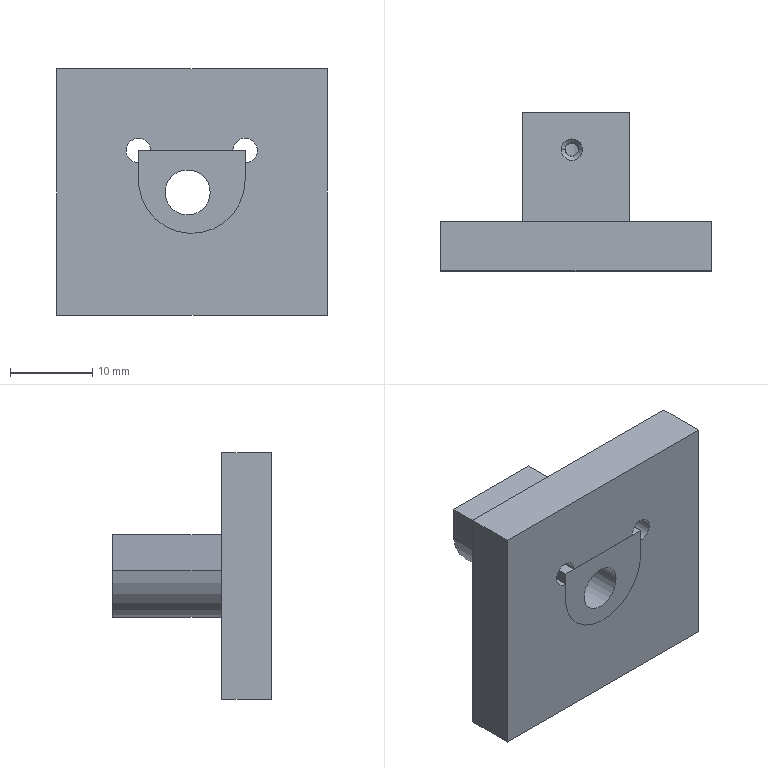Part | NX | 2 solids | 30 faces | box 32.951 x 19.3 x 30.1 mm | volume 6919 mm3 | plane 14 | cylinder 10 | cone 6 | commonest cylinder face diameters 1.6 x4 3 x2 5.5 x2 13 x2
STEP:
#1=CARTESIAN_POINT('',(-6.5,9.65,0.));
#2=VERTEX_POINT('',#1);
#3=CARTESIAN_POINT('',(-6.5,-9.65,0.));
#4=VERTEX_POINT('',#3);
#5=CARTESIAN_POINT('',(-6.5,9.65,0.));
#6=DIRECTION('',(0.,-1.,0.));
#7=VECTOR('',#6,1000.);
#8=LINE('',#5,#7);
#9=EDGE_CURVE('',#2,#4,#8,.T.);
#10=ORIENTED_EDGE('',*,*,#9,.F.);
#11=CARTESIAN_POINT('',(-6.451,9.65,-4.395));
#12=VERTEX_POINT('',#11);
#13=CARTESIAN_POINT('',(-2.87,9.65,-328.33));
#14=DIRECTION('',(0.01106,0.,-0.9999));
#15=VECTOR('',#14,1000.);
#16=LINE('',#13,#15);
#17=EDGE_CURVE('',#2,#12,#16,.T.);
#18=ORIENTED_EDGE('',*,*,#17,.T.);
#19=CARTESIAN_POINT('',(-6.451,-9.65,-4.395));
#20=VERTEX_POINT('',#19);
#21=CARTESIAN_POINT('',(-6.451,9.65,-4.395));
#22=CARTESIAN_POINT('',(-6.451,3.217,-4.395));
#23=CARTESIAN_POINT('',(-6.451,-3.217,-4.395));
#24=CARTESIAN_POINT('',(-6.451,-9.65,-4.395));
#25=B_SPLINE_CURVE_WITH_KNOTS('',3,(#21,#22,#23,#24),.UNSPECIFIED.,.F.,.F.,(4,4),(0.,1.),.UNSPECIFIED.);
#26=EDGE_CURVE('',#20,#12,#25,.F.);
#27=ORIENTED_EDGE('',*,*,#26,.F.);
#28=CARTESIAN_POINT('',(-6.462,-9.65,-3.4));
#29=DIRECTION('',(-0.01106,0.,0.9999));
#30=VECTOR('',#29,1000.);
#31=LINE('',#28,#30);
#32=EDGE_CURVE('',#20,#4,#31,.T.);
#33=ORIENTED_EDGE('',*,*,#32,.T.);
#34=EDGE_LOOP('',(#10,#18,#27,#33));
#35=FACE_BOUND('',#34,.T.);
#36=CARTESIAN_POINT('',(-6.5,-9.65,0.));
#37=DIRECTION('',(-0.9999,0.,-0.01106));
#38=DIRECTION('',(-0.01106,0.,0.9999));
#39=AXIS2_PLACEMENT_3D('',#36,#37,#38);
#40=PLANE('',#39);
#41=ADVANCED_FACE('',(#35),#40,.T.);
#42=ORIENTED_EDGE('',*,*,#32,.F.);
#43=CARTESIAN_POINT('',(6.5,-9.65,-3.6));
#44=VERTEX_POINT('',#43);
#45=CARTESIAN_POINT('',(0.,-9.65,-3.6));
#46=DIRECTION('',(0.,1.,0.));
#47=DIRECTION('',(1.,0.,-0.00002521));
#48=AXIS2_PLACEMENT_3D('',#45,#46,#47);
#49=CIRCLE('',#48,6.5);
#50=EDGE_CURVE('',#44,#20,#49,.T.);
#51=ORIENTED_EDGE('',*,*,#50,.F.);
#52=CARTESIAN_POINT('',(6.5,-9.65,0.));
#53=VERTEX_POINT('',#52);
#54=CARTESIAN_POINT('',(6.5,-9.65,0.));
#55=DIRECTION('',(0.,0.,-1.));
#56=VECTOR('',#55,1000.);
#57=LINE('',#54,#56);
#58=EDGE_CURVE('',#53,#44,#57,.T.);
#59=ORIENTED_EDGE('',*,*,#58,.F.);
#60=CARTESIAN_POINT('',(6.5,-9.65,0.));
#61=DIRECTION('',(-1.,0.,0.));
#62=VECTOR('',#61,1000.);
#63=LINE('',#60,#62);
#64=EDGE_CURVE('',#53,#4,#63,.T.);
#65=ORIENTED_EDGE('',*,*,#64,.T.);
#66=EDGE_LOOP('',(#42,#51,#59,#65));
#67=FACE_BOUND('',#66,.T.);
#68=CARTESIAN_POINT('',(2.25,-9.65,-5.1));
#69=VERTEX_POINT('',#68);
#70=CARTESIAN_POINT('',(-3.25,-9.65,-5.1));
#71=VERTEX_POINT('',#70);
#72=CARTESIAN_POINT('',(-0.5,-9.65,-5.1));
#73=DIRECTION('',(0.,-1.,0.));
#74=DIRECTION('',(1.,0.,0.));
#75=AXIS2_PLACEMENT_3D('',#72,#73,#74);
#76=CIRCLE('',#75,2.75);
#77=EDGE_CURVE('',#69,#71,#76,.T.);
#78=ORIENTED_EDGE('',*,*,#77,.F.);
#79=CARTESIAN_POINT('',(-0.5,-9.65,-5.1));
#80=DIRECTION('',(0.,-1.,0.));
#81=DIRECTION('',(-1.,0.,0.));
#82=AXIS2_PLACEMENT_3D('',#79,#80,#81);
#83=CIRCLE('',#82,2.75);
#84=EDGE_CURVE('',#71,#69,#83,.T.);
#85=ORIENTED_EDGE('',*,*,#84,.F.);
#86=EDGE_LOOP('',(#78,#85));
#87=FACE_BOUND('',#86,.T.);
#88=CARTESIAN_POINT('',(-6.5,-9.65,-3.4));
#89=DIRECTION('',(0.,1.,0.));
#90=DIRECTION('',(-1.,0.,0.));
#91=AXIS2_PLACEMENT_3D('',#88,#89,#90);
#92=PLANE('',#91);
#93=ADVANCED_FACE('',(#67,#87),#92,.F.);
#94=ORIENTED_EDGE('',*,*,#64,.F.);
#95=CARTESIAN_POINT('',(6.5,9.65,0.));
#96=VERTEX_POINT('',#95);
#97=CARTESIAN_POINT('',(6.5,-9.65,0.));
#98=DIRECTION('',(0.,1.,0.));
#99=VECTOR('',#98,1000.);
#100=LINE('',#97,#99);
#101=EDGE_CURVE('',#53,#96,#100,.T.);
#102=ORIENTED_EDGE('',*,*,#101,.T.);
#103=CARTESIAN_POINT('',(-6.5,9.65,0.));
#104=DIRECTION('',(1.,0.,0.));
#105=VECTOR('',#104,1000.);
#106=LINE('',#103,#105);
#107=EDGE_CURVE('',#2,#96,#106,.T.);
#108=ORIENTED_EDGE('',*,*,#107,.F.);
#109=ORIENTED_EDGE('',*,*,#9,.T.);
#110=EDGE_LOOP('',(#94,#102,#108,#109));
#111=FACE_BOUND('',#110,.T.);
#112=CARTESIAN_POINT('',(-0.5,-4.21,0.));
#113=VERTEX_POINT('',#112);
#114=CARTESIAN_POINT('',(-1.8,-5.51,0.));
#115=VERTEX_POINT('',#114);
#116=CARTESIAN_POINT('',(-0.5,-5.51,0.));
#117=DIRECTION('',(0.,0.,1.));
#118=DIRECTION('',(0.,1.,0.));
#119=AXIS2_PLACEMENT_3D('',#116,#117,#118);
#120=CIRCLE('',#119,1.3);
#121=EDGE_CURVE('',#113,#115,#120,.T.);
#122=ORIENTED_EDGE('',*,*,#121,.F.);
#123=CARTESIAN_POINT('',(0.8,-5.51,0.));
#124=VERTEX_POINT('',#123);
#125=CARTESIAN_POINT('',(-0.5,-5.51,0.));
#126=DIRECTION('',(0.,0.,1.));
#127=DIRECTION('',(1.,0.000000004,0.));
#128=AXIS2_PLACEMENT_3D('',#125,#126,#127);
#129=CIRCLE('',#128,1.3);
#130=EDGE_CURVE('',#124,#113,#129,.T.);
#131=ORIENTED_EDGE('',*,*,#130,.F.);
#132=CARTESIAN_POINT('',(-0.5,-6.81,0.));
#133=VERTEX_POINT('',#132);
#134=CARTESIAN_POINT('',(-0.5,-5.51,0.));
#135=DIRECTION('',(0.,0.,1.));
#136=DIRECTION('',(0.,-1.,0.));
#137=AXIS2_PLACEMENT_3D('',#134,#135,#136);
#138=CIRCLE('',#137,1.3);
#139=EDGE_CURVE('',#133,#124,#138,.T.);
#140=ORIENTED_EDGE('',*,*,#139,.F.);
#141=CARTESIAN_POINT('',(-0.5,-5.51,0.));
#142=DIRECTION('',(0.,0.,1.));
#143=DIRECTION('',(-1.,-0.000000004,0.));
#144=AXIS2_PLACEMENT_3D('',#141,#142,#143);
#145=CIRCLE('',#144,1.3);
#146=EDGE_CURVE('',#115,#133,#145,.T.);
#147=ORIENTED_EDGE('',*,*,#146,.F.);
#148=EDGE_LOOP('',(#122,#131,#140,#147));
#149=FACE_BOUND('',#148,.T.);
#150=CARTESIAN_POINT('',(-0.5,6.45,0.));
#151=VERTEX_POINT('',#150);
#152=CARTESIAN_POINT('',(-1.8,5.15,0.));
#153=VERTEX_POINT('',#152);
#154=CARTESIAN_POINT('',(-0.5,5.15,0.));
#155=DIRECTION('',(0.,0.,1.));
#156=DIRECTION('',(0.,1.,0.));
#157=AXIS2_PLACEMENT_3D('',#154,#155,#156);
#158=CIRCLE('',#157,1.3);
#159=EDGE_CURVE('',#151,#153,#158,.T.);
#160=ORIENTED_EDGE('',*,*,#159,.F.);
#161=CARTESIAN_POINT('',(0.8,5.15,0.));
#162=VERTEX_POINT('',#161);
#163=CARTESIAN_POINT('',(-0.5,5.15,0.));
#164=DIRECTION('',(0.,0.,1.));
#165=DIRECTION('',(1.,0.000000004,0.));
#166=AXIS2_PLACEMENT_3D('',#163,#164,#165);
#167=CIRCLE('',#166,1.3);
#168=EDGE_CURVE('',#162,#151,#167,.T.);
#169=ORIENTED_EDGE('',*,*,#168,.F.);
#170=CARTESIAN_POINT('',(-0.5,3.85,0.));
#171=VERTEX_POINT('',#170);
#172=CARTESIAN_POINT('',(-0.5,5.15,0.));
#173=DIRECTION('',(0.,0.,1.));
#174=DIRECTION('',(0.,-1.,0.));
#175=AXIS2_PLACEMENT_3D('',#172,#173,#174);
#176=CIRCLE('',#175,1.3);
#177=EDGE_CURVE('',#171,#162,#176,.T.);
#178=ORIENTED_EDGE('',*,*,#177,.F.);
#179=CARTESIAN_POINT('',(-0.5,5.15,0.));
#180=DIRECTION('',(0.,0.,1.));
#181=DIRECTION('',(-1.,-0.000000004,0.));
#182=AXIS2_PLACEMENT_3D('',#179,#180,#181);
#183=CIRCLE('',#182,1.3);
#184=EDGE_CURVE('',#153,#171,#183,.T.);
#185=ORIENTED_EDGE('',*,*,#184,.F.);
#186=EDGE_LOOP('',(#160,#169,#178,#185));
#187=FACE_BOUND('',#186,.T.);
#188=CARTESIAN_POINT('',(6.5,-9.65,0.));
#189=DIRECTION('',(0.,0.,1.));
#190=DIRECTION('',(1.,0.,0.));
#191=AXIS2_PLACEMENT_3D('',#188,#189,#190);
#192=PLANE('',#191);
#193=ADVANCED_FACE('',(#111,#149,#187),#192,.T.);
#194=CARTESIAN_POINT('',(6.5,9.65,-3.6));
#195=VERTEX_POINT('',#194);
#196=CARTESIAN_POINT('',(6.5,9.65,-3.6));
#197=DIRECTION('',(0.,0.000001693,1.));
#198=VECTOR('',#197,1000.);
#199=LINE('',#196,#198);
#200=EDGE_CURVE('',#195,#96,#199,.T.);
#201=ORIENTED_EDGE('',*,*,#200,.F.);
#202=CARTESIAN_POINT('',(0.,9.65,-3.6));
#203=DIRECTION('',(0.,-1.,0.));
#204=DIRECTION('',(-0.9925,0.,-0.1221));
#205=AXIS2_PLACEMENT_3D('',#202,#203,#204);
#206=CIRCLE('',#205,6.5);
#207=EDGE_CURVE('',#12,#195,#206,.T.);
#208=ORIENTED_EDGE('',*,*,#207,.F.);
#209=ORIENTED_EDGE('',*,*,#17,.F.);
#210=ORIENTED_EDGE('',*,*,#107,.T.);
#211=EDGE_LOOP('',(#201,#208,#209,#210));
#212=FACE_BOUND('',#211,.T.);
#213=CARTESIAN_POINT('',(2.75,9.65,-5.1));
#214=VERTEX_POINT('',#213);
#215=CARTESIAN_POINT('',(-3.75,9.65,-5.1));
#216=VERTEX_POINT('',#215);
#217=CARTESIAN_POINT('',(-0.5,9.65,-5.1));
#218=DIRECTION('',(0.,-1.,0.));
#219=DIRECTION('',(-1.,0.,0.));
#220=AXIS2_PLACEMENT_3D('',#217,#218,#219);
#221=CIRCLE('',#220,3.25);
#222=EDGE_CURVE('',#214,#216,#221,.F.);
#223=ORIENTED_EDGE('',*,*,#222,.F.);
#224=CARTESIAN_POINT('',(-0.5,9.65,-5.1));
#225=DIRECTION('',(0.,-1.,0.));
#226=DIRECTION('',(-1.,0.,0.));
#227=AXIS2_PLACEMENT_3D('',#224,#225,#226);
#228=CIRCLE('',#227,3.25);
#229=EDGE_CURVE('',#216,#214,#228,.F.);
#230=ORIENTED_EDGE('',*,*,#229,.F.);
#231=EDGE_LOOP('',(#223,#230));
#232=FACE_BOUND('',#231,.T.);
#233=CARTESIAN_POINT('',(126.5,9.65,-326.9));
#234=DIRECTION('',(0.,-1.,0.));
#235=DIRECTION('',(1.,0.,0.));
#236=AXIS2_PLACEMENT_3D('',#233,#234,#235);
#237=PLANE('',#236);
#238=ADVANCED_FACE('',(#212,#232),#237,.F.);
#239=ORIENTED_EDGE('',*,*,#207,.T.);
#240=CARTESIAN_POINT('',(6.5,-9.65,-3.6));
#241=DIRECTION('',(0.,1.,-0.000005657));
#242=VECTOR('',#241,1000.);
#243=LINE('',#240,#242);
#244=EDGE_CURVE('',#44,#195,#243,.T.);
#245=ORIENTED_EDGE('',*,*,#244,.F.);
#246=ORIENTED_EDGE('',*,*,#50,.T.);
#247=ORIENTED_EDGE('',*,*,#26,.T.);
#248=EDGE_LOOP('',(#239,#245,#246,#247));
#249=FACE_BOUND('',#248,.T.);
#250=CARTESIAN_POINT('',(0.,-730.231,-3.6));
#251=DIRECTION('',(0.,1.,0.));
#252=DIRECTION('',(-1.,0.,0.));
#253=AXIS2_PLACEMENT_3D('',#250,#251,#252);
#254=CYLINDRICAL_SURFACE('',#253,6.5);
#255=ADVANCED_FACE('',(#249),#254,.T.);
#256=ORIENTED_EDGE('',*,*,#58,.T.);
#257=ORIENTED_EDGE('',*,*,#244,.T.);
#258=ORIENTED_EDGE('',*,*,#200,.T.);
#259=ORIENTED_EDGE('',*,*,#101,.F.);
#260=EDGE_LOOP('',(#256,#257,#258,#259));
#261=FACE_BOUND('',#260,.T.);
#262=CARTESIAN_POINT('',(6.5,-166.75,-133.645));
#263=DIRECTION('',(-1.,0.,0.));
#264=DIRECTION('',(0.,-1.,0.));
#265=AXIS2_PLACEMENT_3D('',#262,#263,#264);
#266=PLANE('',#265);
#267=ADVANCED_FACE('',(#261),#266,.F.);
#268=CARTESIAN_POINT('',(-3.25,9.15,-5.1));
#269=VERTEX_POINT('',#268);
#270=CARTESIAN_POINT('',(-3.25,9.15,-5.1));
#271=CARTESIAN_POINT('',(-3.417,9.317,-5.1));
#272=CARTESIAN_POINT('',(-3.556,9.456,-5.1));
#273=CARTESIAN_POINT('',(-3.75,9.65,-5.1));
#274=B_SPLINE_CURVE_WITH_KNOTS('',3,(#270,#271,#272,#273),.UNSPECIFIED.,.F.,.F.,(4,4),(0.,0.9998),.UNSPECIFIED.);
#275=EDGE_CURVE('',#269,#216,#274,.T.);
#276=ORIENTED_EDGE('',*,*,#275,.T.);
#277=ORIENTED_EDGE('',*,*,#229,.T.);
#278=CARTESIAN_POINT('',(2.25,9.15,-5.1));
#279=VERTEX_POINT('',#278);
#280=CARTESIAN_POINT('',(2.75,9.65,-5.1));
#281=CARTESIAN_POINT('',(2.583,9.483,-5.1));
#282=CARTESIAN_POINT('',(2.416,9.317,-5.1));
#283=CARTESIAN_POINT('',(2.25,9.15,-5.1));
#284=B_SPLINE_CURVE_WITH_KNOTS('',3,(#280,#281,#282,#283),.UNSPECIFIED.,.F.,.F.,(4,4),(0.0001808,1.),.UNSPECIFIED.);
#285=EDGE_CURVE('',#214,#279,#284,.T.);
#286=ORIENTED_EDGE('',*,*,#285,.T.);
#287=CARTESIAN_POINT('',(-0.5,9.15,-5.1));
#288=DIRECTION('',(0.,1.,0.));
#289=DIRECTION('',(1.,0.,0.));
#290=AXIS2_PLACEMENT_3D('',#287,#288,#289);
#291=CIRCLE('',#290,2.75);
#292=EDGE_CURVE('',#269,#279,#291,.T.);
#293=ORIENTED_EDGE('',*,*,#292,.F.);
#294=EDGE_LOOP('',(#276,#277,#286,#293));
#295=FACE_BOUND('',#294,.T.);
#296=CARTESIAN_POINT('',(-0.5,9.4,-5.1));
#297=DIRECTION('',(0.,1.,0.));
#298=DIRECTION('',(-1.,0.,0.));
#299=AXIS2_PLACEMENT_3D('',#296,#297,#298);
#300=CONICAL_SURFACE('',#299,3.,0.7853);
#301=ADVANCED_FACE('',(#295),#300,.F.);
#302=CARTESIAN_POINT('',(2.25,-244.,-5.1));
#303=DIRECTION('',(0.,-1.,0.));
#304=VECTOR('',#303,1000.);
#305=LINE('',#302,#304);
#306=EDGE_CURVE('',#69,#279,#305,.F.);
#307=ORIENTED_EDGE('',*,*,#306,.F.);
#308=ORIENTED_EDGE('',*,*,#77,.T.);
#309=CARTESIAN_POINT('',(-3.25,-244.,-5.1));
#310=DIRECTION('',(0.,-1.,0.));
#311=VECTOR('',#310,1000.);
#312=LINE('',#309,#311);
#313=EDGE_CURVE('',#71,#269,#312,.F.);
#314=ORIENTED_EDGE('',*,*,#313,.T.);
#315=ORIENTED_EDGE('',*,*,#292,.T.);
#316=EDGE_LOOP('',(#307,#308,#314,#315));
#317=FACE_BOUND('',#316,.T.);
#318=CARTESIAN_POINT('',(-1.3,-5.51,-2.469));
#319=VERTEX_POINT('',#318);
#320=CARTESIAN_POINT('',(0.3,-5.51,-2.469));
#321=VERTEX_POINT('',#320);
#322=CARTESIAN_POINT('',(-1.3,-5.51,-2.469));
#323=CARTESIAN_POINT('',(-1.3,-5.085,-2.469));
#324=CARTESIAN_POINT('',(-0.5015,-4.336,-2.231));
#325=CARTESIAN_POINT('',(0.3,-5.085,-2.469));
#326=CARTESIAN_POINT('',(0.3,-5.51,-2.469));
#327=B_SPLINE_CURVE_WITH_KNOTS('',3,(#322,#323,#324,#325,#326),.UNSPECIFIED.,.F.,.F.,(4,1,4),(0.,0.001257,0.002514),.UNSPECIFIED.);
#328=EDGE_CURVE('',#319,#321,#327,.T.);
#329=ORIENTED_EDGE('',*,*,#328,.F.);
#330=CARTESIAN_POINT('',(0.3,-5.51,-2.469));
#331=CARTESIAN_POINT('',(0.3,-5.936,-2.469));
#332=CARTESIAN_POINT('',(-0.4985,-6.685,-2.231));
#333=CARTESIAN_POINT('',(-1.3,-5.936,-2.469));
#334=CARTESIAN_POINT('',(-1.3,-5.51,-2.469));
#335=B_SPLINE_CURVE_WITH_KNOTS('',3,(#330,#331,#332,#333,#334),.UNSPECIFIED.,.F.,.F.,(4,1,4),(0.,0.001257,0.002514),.UNSPECIFIED.);
#336=EDGE_CURVE('',#321,#319,#335,.T.);
#337=ORIENTED_EDGE('',*,*,#336,.F.);
#338=EDGE_LOOP('',(#329,#337));
#339=FACE_BOUND('',#338,.T.);
#340=CARTESIAN_POINT('',(-1.3,5.15,-2.469));
#341=VERTEX_POINT('',#340);
#342=CARTESIAN_POINT('',(0.3,5.15,-2.469));
#343=VERTEX_POINT('',#342);
#344=CARTESIAN_POINT('',(-1.3,5.15,-2.469));
#345=CARTESIAN_POINT('',(-1.3,5.575,-2.469));
#346=CARTESIAN_POINT('',(-0.5015,6.325,-2.231));
#347=CARTESIAN_POINT('',(0.3,5.575,-2.469));
#348=CARTESIAN_POINT('',(0.3,5.15,-2.469));
#349=B_SPLINE_CURVE_WITH_KNOTS('',3,(#344,#345,#346,#347,#348),.UNSPECIFIED.,.F.,.F.,(4,1,4),(0.,0.001257,0.002514),.UNSPECIFIED.);
#350=EDGE_CURVE('',#341,#343,#349,.T.);
#351=ORIENTED_EDGE('',*,*,#350,.F.);
#352=CARTESIAN_POINT('',(0.3,5.15,-2.469));
#353=CARTESIAN_POINT('',(0.3,4.725,-2.469));
#354=CARTESIAN_POINT('',(-0.4985,3.975,-2.231));
#355=CARTESIAN_POINT('',(-1.3,4.725,-2.469));
#356=CARTESIAN_POINT('',(-1.3,5.15,-2.469));
#357=B_SPLINE_CURVE_WITH_KNOTS('',3,(#352,#353,#354,#355,#356),.UNSPECIFIED.,.F.,.F.,(4,1,4),(0.,0.001257,0.002514),.UNSPECIFIED.);
#358=EDGE_CURVE('',#343,#341,#357,.T.);
#359=ORIENTED_EDGE('',*,*,#358,.F.);
#360=EDGE_LOOP('',(#351,#359));
#361=FACE_BOUND('',#360,.T.);
#362=CARTESIAN_POINT('',(-0.5,-244.,-5.1));
#363=DIRECTION('',(0.,-1.,0.));
#364=DIRECTION('',(1.,0.,0.));
#365=AXIS2_PLACEMENT_3D('',#362,#363,#364);
#366=CYLINDRICAL_SURFACE('',#365,2.75);
#367=ADVANCED_FACE('',(#317,#339,#361),#366,.F.);
#368=CARTESIAN_POINT('',(-0.5,9.15,-5.1));
#369=DIRECTION('',(0.,1.,0.));
#370=DIRECTION('',(1.,0.,0.));
#371=AXIS2_PLACEMENT_3D('',#368,#369,#370);
#372=CIRCLE('',#371,2.75);
#373=EDGE_CURVE('',#279,#269,#372,.T.);
#374=ORIENTED_EDGE('',*,*,#373,.T.);
#375=ORIENTED_EDGE('',*,*,#313,.F.);
#376=ORIENTED_EDGE('',*,*,#84,.T.);
#377=ORIENTED_EDGE('',*,*,#306,.T.);
#378=EDGE_LOOP('',(#374,#375,#376,#377));
#379=FACE_BOUND('',#378,.T.);
#380=CARTESIAN_POINT('',(-0.5,-244.,-5.1));
#381=DIRECTION('',(0.,-1.,0.));
#382=DIRECTION('',(1.,0.,0.));
#383=AXIS2_PLACEMENT_3D('',#380,#381,#382);
#384=CYLINDRICAL_SURFACE('',#383,2.75);
#385=ADVANCED_FACE('',(#379),#384,.F.);
#386=ORIENTED_EDGE('',*,*,#285,.F.);
#387=ORIENTED_EDGE('',*,*,#222,.T.);
#388=ORIENTED_EDGE('',*,*,#275,.F.);
#389=ORIENTED_EDGE('',*,*,#373,.F.);
#390=EDGE_LOOP('',(#386,#387,#388,#389));
#391=FACE_BOUND('',#390,.T.);
#392=CARTESIAN_POINT('',(-0.5,9.4,-5.1));
#393=DIRECTION('',(0.,1.,0.));
#394=DIRECTION('',(-1.,0.,0.));
#395=AXIS2_PLACEMENT_3D('',#392,#393,#394);
#396=CONICAL_SURFACE('',#395,3.,0.7853);
#397=ADVANCED_FACE('',(#391),#396,.F.);
#398=CARTESIAN_POINT('',(0.3,-5.51,-0.5));
#399=VERTEX_POINT('',#398);
#400=CARTESIAN_POINT('',(0.3,-5.51,-2.469));
#401=DIRECTION('',(0.000000004,0.000000196,1.));
#402=VECTOR('',#401,1000.);
#403=LINE('',#400,#402);
#404=EDGE_CURVE('',#399,#321,#403,.F.);
#405=ORIENTED_EDGE('',*,*,#404,.T.);
#406=ORIENTED_EDGE('',*,*,#336,.T.);
#407=CARTESIAN_POINT('',(-1.3,-5.51,-0.5));
#408=VERTEX_POINT('',#407);
#409=CARTESIAN_POINT('',(-1.3,-5.51,-2.469));
#410=DIRECTION('',(-0.000000004,-0.000000157,1.));
#411=VECTOR('',#410,1000.);
#412=LINE('',#409,#411);
#413=EDGE_CURVE('',#408,#319,#412,.F.);
#414=ORIENTED_EDGE('',*,*,#413,.F.);
#415=CARTESIAN_POINT('',(-0.5,-6.31,-0.5));
#416=VERTEX_POINT('',#415);
#417=CARTESIAN_POINT('',(-0.5,-5.51,-0.5));
#418=DIRECTION('',(0.,0.,1.));
#419=DIRECTION('',(-1.,0.,0.));
#420=AXIS2_PLACEMENT_3D('',#417,#418,#419);
#421=CIRCLE('',#420,0.8);
#422=EDGE_CURVE('',#408,#416,#421,.T.);
#423=ORIENTED_EDGE('',*,*,#422,.T.);
#424=CARTESIAN_POINT('',(-0.5,-5.51,-0.5));
#425=DIRECTION('',(0.,0.,1.));
#426=DIRECTION('',(0.,-1.,0.));
#427=AXIS2_PLACEMENT_3D('',#424,#425,#426);
#428=CIRCLE('',#427,0.8);
#429=EDGE_CURVE('',#416,#399,#428,.T.);
#430=ORIENTED_EDGE('',*,*,#429,.T.);
#431=EDGE_LOOP('',(#405,#406,#414,#423,#430));
#432=FACE_BOUND('',#431,.T.);
#433=CARTESIAN_POINT('',(-0.5,-5.51,1.1));
#434=DIRECTION('',(0.,0.,1.));
#435=DIRECTION('',(1.,0.,0.));
#436=AXIS2_PLACEMENT_3D('',#433,#434,#435);
#437=CYLINDRICAL_SURFACE('',#436,0.8);
#438=ADVANCED_FACE('',(#432),#437,.F.);
#439=CARTESIAN_POINT('',(0.8,-5.51,0.));
#440=DIRECTION('',(-0.7071,-0.000000331,-0.7071));
#441=VECTOR('',#440,1000.);
#442=LINE('',#439,#441);
#443=EDGE_CURVE('',#399,#124,#442,.F.);
#444=ORIENTED_EDGE('',*,*,#443,.F.);
#445=ORIENTED_EDGE('',*,*,#429,.F.);
#446=ORIENTED_EDGE('',*,*,#422,.F.);
#447=CARTESIAN_POINT('',(-1.8,-5.51,0.));
#448=DIRECTION('',(0.7071,0.000000005,-0.7071));
#449=VECTOR('',#448,1000.);
#450=LINE('',#447,#449);
#451=EDGE_CURVE('',#408,#115,#450,.F.);
#452=ORIENTED_EDGE('',*,*,#451,.T.);
#453=ORIENTED_EDGE('',*,*,#146,.T.);
#454=ORIENTED_EDGE('',*,*,#139,.T.);
#455=EDGE_LOOP('',(#444,#445,#446,#452,#453,#454));
#456=FACE_BOUND('',#455,.T.);
#457=CARTESIAN_POINT('',(-0.5,-5.51,-0.25));
#458=DIRECTION('',(0.,0.,1.));
#459=DIRECTION('',(0.,-1.,0.));
#460=AXIS2_PLACEMENT_3D('',#457,#458,#459);
#461=CONICAL_SURFACE('',#460,1.05,0.7854);
#462=ADVANCED_FACE('',(#456),#461,.F.);
#463=ORIENTED_EDGE('',*,*,#451,.F.);
#464=CARTESIAN_POINT('',(-0.5,-4.71,-0.5));
#465=VERTEX_POINT('',#464);
#466=CARTESIAN_POINT('',(-0.5,-5.51,-0.5));
#467=DIRECTION('',(0.,0.,1.));
#468=DIRECTION('',(0.,1.,0.));
#469=AXIS2_PLACEMENT_3D('',#466,#467,#468);
#470=CIRCLE('',#469,0.8);
#471=EDGE_CURVE('',#465,#408,#470,.T.);
#472=ORIENTED_EDGE('',*,*,#471,.F.);
#473=CARTESIAN_POINT('',(-0.5,-5.51,-0.5));
#474=DIRECTION('',(0.,0.,1.));
#475=DIRECTION('',(1.,-0.000000577,0.));
#476=AXIS2_PLACEMENT_3D('',#473,#474,#475);
#477=CIRCLE('',#476,0.8);
#478=EDGE_CURVE('',#399,#465,#477,.T.);
#479=ORIENTED_EDGE('',*,*,#478,.F.);
#480=ORIENTED_EDGE('',*,*,#443,.T.);
#481=ORIENTED_EDGE('',*,*,#130,.T.);
#482=ORIENTED_EDGE('',*,*,#121,.T.);
#483=EDGE_LOOP('',(#463,#472,#479,#480,#481,#482));
#484=FACE_BOUND('',#483,.T.);
#485=CARTESIAN_POINT('',(-0.5,-5.51,-0.25));
#486=DIRECTION('',(0.,0.,1.));
#487=DIRECTION('',(0.,-1.,0.));
#488=AXIS2_PLACEMENT_3D('',#485,#486,#487);
#489=CONICAL_SURFACE('',#488,1.05,0.7854);
#490=ADVANCED_FACE('',(#484),#489,.F.);
#491=ORIENTED_EDGE('',*,*,#413,.T.);
#492=ORIENTED_EDGE('',*,*,#328,.T.);
#493=ORIENTED_EDGE('',*,*,#404,.F.);
#494=ORIENTED_EDGE('',*,*,#478,.T.);
#495=ORIENTED_EDGE('',*,*,#471,.T.);
#496=EDGE_LOOP('',(#491,#492,#493,#494,#495));
#497=FACE_BOUND('',#496,.T.);
#498=CARTESIAN_POINT('',(-0.5,-5.51,1.1));
#499=DIRECTION('',(0.,0.,1.));
#500=DIRECTION('',(1.,0.,0.));
#501=AXIS2_PLACEMENT_3D('',#498,#499,#500);
#502=CYLINDRICAL_SURFACE('',#501,0.8);
#503=ADVANCED_FACE('',(#497),#502,.F.);
#504=CARTESIAN_POINT('',(0.3,5.15,-0.5));
#505=VERTEX_POINT('',#504);
#506=CARTESIAN_POINT('',(0.3,5.15,-2.469));
#507=DIRECTION('',(0.000000004,0.000000196,1.));
#508=VECTOR('',#507,1000.);
#509=LINE('',#506,#508);
#510=EDGE_CURVE('',#505,#343,#509,.F.);
#511=ORIENTED_EDGE('',*,*,#510,.T.);
#512=ORIENTED_EDGE('',*,*,#358,.T.);
#513=CARTESIAN_POINT('',(-1.3,5.15,-0.5));
#514=VERTEX_POINT('',#513);
#515=CARTESIAN_POINT('',(-1.3,5.15,-2.469));
#516=DIRECTION('',(-0.000000004,-0.000000157,1.));
#517=VECTOR('',#516,1000.);
#518=LINE('',#515,#517);
#519=EDGE_CURVE('',#514,#341,#518,.F.);
#520=ORIENTED_EDGE('',*,*,#519,.F.);
#521=CARTESIAN_POINT('',(-0.5,4.35,-0.5));
#522=VERTEX_POINT('',#521);
#523=CARTESIAN_POINT('',(-0.5,5.15,-0.5));
#524=DIRECTION('',(0.,0.,1.));
#525=DIRECTION('',(-1.,0.,0.));
#526=AXIS2_PLACEMENT_3D('',#523,#524,#525);
#527=CIRCLE('',#526,0.8);
#528=EDGE_CURVE('',#514,#522,#527,.T.);
#529=ORIENTED_EDGE('',*,*,#528,.T.);
#530=CARTESIAN_POINT('',(-0.5,5.15,-0.5));
#531=DIRECTION('',(0.,0.,1.));
#532=DIRECTION('',(0.,-1.,0.));
#533=AXIS2_PLACEMENT_3D('',#530,#531,#532);
#534=CIRCLE('',#533,0.8);
#535=EDGE_CURVE('',#522,#505,#534,.T.);
#536=ORIENTED_EDGE('',*,*,#535,.T.);
#537=EDGE_LOOP('',(#511,#512,#520,#529,#536));
#538=FACE_BOUND('',#537,.T.);
#539=CARTESIAN_POINT('',(-0.5,5.15,1.1));
#540=DIRECTION('',(0.,0.,1.));
#541=DIRECTION('',(1.,0.,0.));
#542=AXIS2_PLACEMENT_3D('',#539,#540,#541);
#543=CYLINDRICAL_SURFACE('',#542,0.8);
#544=ADVANCED_FACE('',(#538),#543,.F.);
#545=CARTESIAN_POINT('',(0.8,5.15,0.));
#546=DIRECTION('',(-0.7071,-0.000000331,-0.7071));
#547=VECTOR('',#546,1000.);
#548=LINE('',#545,#547);
#549=EDGE_CURVE('',#505,#162,#548,.F.);
#550=ORIENTED_EDGE('',*,*,#549,.F.);
#551=ORIENTED_EDGE('',*,*,#535,.F.);
#552=ORIENTED_EDGE('',*,*,#528,.F.);
#553=CARTESIAN_POINT('',(-1.8,5.15,0.));
#554=DIRECTION('',(0.7071,0.000000005,-0.7071));
#555=VECTOR('',#554,1000.);
#556=LINE('',#553,#555);
#557=EDGE_CURVE('',#514,#153,#556,.F.);
#558=ORIENTED_EDGE('',*,*,#557,.T.);
#559=ORIENTED_EDGE('',*,*,#184,.T.);
#560=ORIENTED_EDGE('',*,*,#177,.T.);
#561=EDGE_LOOP('',(#550,#551,#552,#558,#559,#560));
#562=FACE_BOUND('',#561,.T.);
#563=CARTESIAN_POINT('',(-0.5,5.15,-0.25));
#564=DIRECTION('',(0.,0.,1.));
#565=DIRECTION('',(0.,-1.,0.));
#566=AXIS2_PLACEMENT_3D('',#563,#564,#565);
#567=CONICAL_SURFACE('',#566,1.05,0.7854);
#568=ADVANCED_FACE('',(#562),#567,.F.);
#569=ORIENTED_EDGE('',*,*,#557,.F.);
#570=CARTESIAN_POINT('',(-0.5,5.95,-0.5));
#571=VERTEX_POINT('',#570);
#572=CARTESIAN_POINT('',(-0.5,5.15,-0.5));
#573=DIRECTION('',(0.,0.,1.));
#574=DIRECTION('',(0.,1.,0.));
#575=AXIS2_PLACEMENT_3D('',#572,#573,#574);
#576=CIRCLE('',#575,0.8);
#577=EDGE_CURVE('',#571,#514,#576,.T.);
#578=ORIENTED_EDGE('',*,*,#577,.F.);
#579=CARTESIAN_POINT('',(-0.5,5.15,-0.5));
#580=DIRECTION('',(0.,0.,1.));
#581=DIRECTION('',(1.,-0.000000577,0.));
#582=AXIS2_PLACEMENT_3D('',#579,#580,#581);
#583=CIRCLE('',#582,0.8);
#584=EDGE_CURVE('',#505,#571,#583,.T.);
#585=ORIENTED_EDGE('',*,*,#584,.F.);
#586=ORIENTED_EDGE('',*,*,#549,.T.);
#587=ORIENTED_EDGE('',*,*,#168,.T.);
#588=ORIENTED_EDGE('',*,*,#159,.T.);
#589=EDGE_LOOP('',(#569,#578,#585,#586,#587,#588));
#590=FACE_BOUND('',#589,.T.);
#591=CARTESIAN_POINT('',(-0.5,5.15,-0.25));
#592=DIRECTION('',(0.,0.,1.));
#593=DIRECTION('',(0.,-1.,0.));
#594=AXIS2_PLACEMENT_3D('',#591,#592,#593);
#595=CONICAL_SURFACE('',#594,1.05,0.7854);
#596=ADVANCED_FACE('',(#590),#595,.F.);
#597=ORIENTED_EDGE('',*,*,#519,.T.);
#598=ORIENTED_EDGE('',*,*,#350,.T.);
#599=ORIENTED_EDGE('',*,*,#510,.F.);
#600=ORIENTED_EDGE('',*,*,#584,.T.);
#601=ORIENTED_EDGE('',*,*,#577,.T.);
#602=EDGE_LOOP('',(#597,#598,#599,#600,#601));
#603=FACE_BOUND('',#602,.T.);
#604=CARTESIAN_POINT('',(-0.5,5.15,1.1));
#605=DIRECTION('',(0.,0.,1.));
#606=DIRECTION('',(1.,0.,0.));
#607=AXIS2_PLACEMENT_3D('',#604,#605,#606);
#608=CYLINDRICAL_SURFACE('',#607,0.8);
#609=ADVANCED_FACE('',(#603),#608,.F.);
#610=CLOSED_SHELL('',(#41,#93,#193,#238,#255,#267,#301,#367,#385,#397,#438,#462,#490,#503,#544,#568,#596,#609));
#611=MANIFOLD_SOLID_BREP('',#610);
#612=CARTESIAN_POINT('',(-6.451,-9.65,-4.395));
#613=VERTEX_POINT('',#612);
#614=CARTESIAN_POINT('',(6.5,-9.65,-3.6));
#615=VERTEX_POINT('',#614);
#616=CARTESIAN_POINT('',(0.,-9.65,-3.6));
#617=DIRECTION('',(0.,-1.,0.));
#618=DIRECTION('',(1.,0.,-0.00002521));
#619=AXIS2_PLACEMENT_3D('',#616,#617,#618);
#620=CIRCLE('',#619,6.5);
#621=EDGE_CURVE('',#613,#615,#620,.T.);
#622=ORIENTED_EDGE('',*,*,#621,.T.);
#623=CARTESIAN_POINT('',(6.5,-3.65,-3.6));
#624=VERTEX_POINT('',#623);
#625=CARTESIAN_POINT('',(6.5,-3.65,-3.6));
#626=DIRECTION('',(0.,-1.,0.));
#627=VECTOR('',#626,1000.);
#628=LINE('',#625,#627);
#629=EDGE_CURVE('',#624,#615,#628,.T.);
#630=ORIENTED_EDGE('',*,*,#629,.F.);
#631=CARTESIAN_POINT('',(-6.451,-3.65,-4.395));
#632=VERTEX_POINT('',#631);
#633=CARTESIAN_POINT('',(0.,-3.65,-3.6));
#634=DIRECTION('',(0.,-1.,0.));
#635=DIRECTION('',(1.,0.,-0.00002521));
#636=AXIS2_PLACEMENT_3D('',#633,#634,#635);
#637=CIRCLE('',#636,6.5);
#638=EDGE_CURVE('',#632,#624,#637,.T.);
#639=ORIENTED_EDGE('',*,*,#638,.F.);
#640=CARTESIAN_POINT('',(-6.451,-9.65,-4.395));
#641=CARTESIAN_POINT('',(-6.451,-7.65,-4.395));
#642=CARTESIAN_POINT('',(-6.451,-5.65,-4.395));
#643=CARTESIAN_POINT('',(-6.451,-3.65,-4.395));
#644=B_SPLINE_CURVE_WITH_KNOTS('',3,(#640,#641,#642,#643),.UNSPECIFIED.,.F.,.F.,(4,4),(0.,1.),.UNSPECIFIED.);
#645=EDGE_CURVE('',#632,#613,#644,.F.);
#646=ORIENTED_EDGE('',*,*,#645,.T.);
#647=EDGE_LOOP('',(#622,#630,#639,#646));
#648=FACE_BOUND('',#647,.T.);
#649=CARTESIAN_POINT('',(0.,-3.65,-3.6));
#650=DIRECTION('',(0.,-1.,0.));
#651=DIRECTION('',(0.,0.,-1.));
#652=AXIS2_PLACEMENT_3D('',#649,#650,#651);
#653=CYLINDRICAL_SURFACE('',#652,6.5);
#654=ADVANCED_FACE('',(#648),#653,.F.);
#655=CARTESIAN_POINT('',(6.5,-9.65,-1.5));
#656=VERTEX_POINT('',#655);
#657=CARTESIAN_POINT('',(6.5,-9.65,-3.6));
#658=DIRECTION('',(0.,0.,1.));
#659=VECTOR('',#658,1000.);
#660=LINE('',#657,#659);
#661=EDGE_CURVE('',#615,#656,#660,.T.);
#662=ORIENTED_EDGE('',*,*,#661,.T.);
#663=CARTESIAN_POINT('',(6.5,-3.65,-1.5));
#664=VERTEX_POINT('',#663);
#665=CARTESIAN_POINT('',(6.5,-3.65,-1.5));
#666=DIRECTION('',(0.,-1.,0.));
#667=VECTOR('',#666,1000.);
#668=LINE('',#665,#667);
#669=EDGE_CURVE('',#664,#656,#668,.T.);
#670=ORIENTED_EDGE('',*,*,#669,.F.);
#671=CARTESIAN_POINT('',(6.5,-3.65,-3.6));
#672=DIRECTION('',(0.,0.,1.));
#673=VECTOR('',#672,1000.);
#674=LINE('',#671,#673);
#675=EDGE_CURVE('',#624,#664,#674,.T.);
#676=ORIENTED_EDGE('',*,*,#675,.F.);
#677=ORIENTED_EDGE('',*,*,#629,.T.);
#678=EDGE_LOOP('',(#662,#670,#676,#677));
#679=FACE_BOUND('',#678,.T.);
#680=CARTESIAN_POINT('',(6.5,-3.65,-3.6));
#681=DIRECTION('',(1.,0.,0.));
#682=DIRECTION('',(0.,0.,-1.));
#683=AXIS2_PLACEMENT_3D('',#680,#681,#682);
#684=PLANE('',#683);
#685=ADVANCED_FACE('',(#679),#684,.F.);
#686=CARTESIAN_POINT('',(5.,-9.65,0.));
#687=VERTEX_POINT('',#686);
#688=CARTESIAN_POINT('',(6.5,-9.65,0.));
#689=DIRECTION('',(0.,-1.,0.));
#690=DIRECTION('',(0.,0.,-1.));
#691=AXIS2_PLACEMENT_3D('',#688,#689,#690);
#692=CIRCLE('',#691,1.5);
#693=EDGE_CURVE('',#656,#687,#692,.T.);
#694=ORIENTED_EDGE('',*,*,#693,.T.);
#695=CARTESIAN_POINT('',(5.,-3.65,0.));
#696=VERTEX_POINT('',#695);
#697=CARTESIAN_POINT('',(5.,-3.65,0.));
#698=DIRECTION('',(0.,-1.,0.));
#699=VECTOR('',#698,1000.);
#700=LINE('',#697,#699);
#701=EDGE_CURVE('',#696,#687,#700,.T.);
#702=ORIENTED_EDGE('',*,*,#701,.F.);
#703=CARTESIAN_POINT('',(6.5,-3.65,0.));
#704=DIRECTION('',(0.,-1.,0.));
#705=DIRECTION('',(0.,0.,-1.));
#706=AXIS2_PLACEMENT_3D('',#703,#704,#705);
#707=CIRCLE('',#706,1.5);
#708=EDGE_CURVE('',#664,#696,#707,.T.);
#709=ORIENTED_EDGE('',*,*,#708,.F.);
#710=ORIENTED_EDGE('',*,*,#669,.T.);
#711=EDGE_LOOP('',(#694,#702,#709,#710));
#712=FACE_BOUND('',#711,.T.);
#713=CARTESIAN_POINT('',(6.5,-3.65,0.));
#714=DIRECTION('',(0.,-1.,0.));
#715=DIRECTION('',(0.,0.,-1.));
#716=AXIS2_PLACEMENT_3D('',#713,#714,#715);
#717=CYLINDRICAL_SURFACE('',#716,1.5);
#718=ADVANCED_FACE('',(#712),#717,.F.);
#719=CARTESIAN_POINT('',(-5.,-9.65,0.));
#720=VERTEX_POINT('',#719);
#721=CARTESIAN_POINT('',(5.,-9.65,0.));
#722=DIRECTION('',(-1.,0.,0.));
#723=VECTOR('',#722,1000.);
#724=LINE('',#721,#723);
#725=EDGE_CURVE('',#687,#720,#724,.T.);
#726=ORIENTED_EDGE('',*,*,#725,.T.);
#727=CARTESIAN_POINT('',(-5.,-3.65,0.));
#728=VERTEX_POINT('',#727);
#729=CARTESIAN_POINT('',(-5.,-3.65,0.));
#730=DIRECTION('',(0.,-1.,0.));
#731=VECTOR('',#730,1000.);
#732=LINE('',#729,#731);
#733=EDGE_CURVE('',#728,#720,#732,.T.);
#734=ORIENTED_EDGE('',*,*,#733,.F.);
#735=CARTESIAN_POINT('',(5.,-3.65,0.));
#736=DIRECTION('',(-1.,0.,0.));
#737=VECTOR('',#736,1000.);
#738=LINE('',#735,#737);
#739=EDGE_CURVE('',#696,#728,#738,.T.);
#740=ORIENTED_EDGE('',*,*,#739,.F.);
#741=ORIENTED_EDGE('',*,*,#701,.T.);
#742=EDGE_LOOP('',(#726,#734,#740,#741));
#743=FACE_BOUND('',#742,.T.);
#744=CARTESIAN_POINT('',(5.,-3.65,0.));
#745=DIRECTION('',(0.,0.,1.));
#746=DIRECTION('',(1.,0.,0.));
#747=AXIS2_PLACEMENT_3D('',#744,#745,#746);
#748=PLANE('',#747);
#749=ADVANCED_FACE('',(#743),#748,.F.);
#750=CARTESIAN_POINT('',(-6.483,-9.65,-1.5));
#751=VERTEX_POINT('',#750);
#752=CARTESIAN_POINT('',(-6.5,-9.65,0.));
#753=DIRECTION('',(0.,-1.,0.));
#754=DIRECTION('',(0.,0.,-1.));
#755=AXIS2_PLACEMENT_3D('',#752,#753,#754);
#756=CIRCLE('',#755,1.5);
#757=EDGE_CURVE('',#720,#751,#756,.T.);
#758=ORIENTED_EDGE('',*,*,#757,.T.);
#759=CARTESIAN_POINT('',(-6.483,-3.65,-1.5));
#760=VERTEX_POINT('',#759);
#761=CARTESIAN_POINT('',(-6.483,-3.65,-1.5));
#762=DIRECTION('',(0.,-1.,0.));
#763=VECTOR('',#762,1000.);
#764=LINE('',#761,#763);
#765=EDGE_CURVE('',#760,#751,#764,.T.);
#766=ORIENTED_EDGE('',*,*,#765,.F.);
#767=CARTESIAN_POINT('',(-6.5,-3.65,0.));
#768=DIRECTION('',(0.,-1.,0.));
#769=DIRECTION('',(0.,0.,-1.));
#770=AXIS2_PLACEMENT_3D('',#767,#768,#769);
#771=CIRCLE('',#770,1.5);
#772=EDGE_CURVE('',#728,#760,#771,.T.);
#773=ORIENTED_EDGE('',*,*,#772,.F.);
#774=ORIENTED_EDGE('',*,*,#733,.T.);
#775=EDGE_LOOP('',(#758,#766,#773,#774));
#776=FACE_BOUND('',#775,.T.);
#777=CARTESIAN_POINT('',(-6.5,-3.65,0.));
#778=DIRECTION('',(0.,-1.,0.));
#779=DIRECTION('',(0.,0.,-1.));
#780=AXIS2_PLACEMENT_3D('',#777,#778,#779);
#781=CYLINDRICAL_SURFACE('',#780,1.5);
#782=ADVANCED_FACE('',(#776),#781,.F.);
#783=CARTESIAN_POINT('',(-16.451,-9.65,10.));
#784=VERTEX_POINT('',#783);
#785=CARTESIAN_POINT('',(16.5,-9.65,10.));
#786=VERTEX_POINT('',#785);
#787=CARTESIAN_POINT('',(-16.451,-9.65,10.));
#788=DIRECTION('',(1.,0.,0.));
#789=VECTOR('',#788,1000.);
#790=LINE('',#787,#789);
#791=EDGE_CURVE('',#784,#786,#790,.T.);
#792=ORIENTED_EDGE('',*,*,#791,.T.);
#793=CARTESIAN_POINT('',(16.5,-3.65,10.));
#794=VERTEX_POINT('',#793);
#795=CARTESIAN_POINT('',(16.5,-3.65,10.));
#796=DIRECTION('',(0.,-1.,0.));
#797=VECTOR('',#796,1000.);
#798=LINE('',#795,#797);
#799=EDGE_CURVE('',#794,#786,#798,.T.);
#800=ORIENTED_EDGE('',*,*,#799,.F.);
#801=CARTESIAN_POINT('',(-16.451,-3.65,10.));
#802=VERTEX_POINT('',#801);
#803=CARTESIAN_POINT('',(-16.451,-3.65,10.));
#804=DIRECTION('',(1.,0.,0.));
#805=VECTOR('',#804,1000.);
#806=LINE('',#803,#805);
#807=EDGE_CURVE('',#802,#794,#806,.T.);
#808=ORIENTED_EDGE('',*,*,#807,.F.);
#809=CARTESIAN_POINT('',(-16.451,-3.65,10.));
#810=DIRECTION('',(0.,-1.,0.));
#811=VECTOR('',#810,1000.);
#812=LINE('',#809,#811);
#813=EDGE_CURVE('',#802,#784,#812,.T.);
#814=ORIENTED_EDGE('',*,*,#813,.T.);
#815=EDGE_LOOP('',(#792,#800,#808,#814));
#816=FACE_BOUND('',#815,.T.);
#817=CARTESIAN_POINT('',(-16.451,-3.65,10.));
#818=DIRECTION('',(0.,0.,-1.));
#819=DIRECTION('',(-1.,0.,0.));
#820=AXIS2_PLACEMENT_3D('',#817,#818,#819);
#821=PLANE('',#820);
#822=ADVANCED_FACE('',(#816),#821,.F.);
#823=CARTESIAN_POINT('',(16.5,-9.65,-20.1));
#824=VERTEX_POINT('',#823);
#825=CARTESIAN_POINT('',(16.5,-9.65,10.));
#826=DIRECTION('',(0.,0.,-1.));
#827=VECTOR('',#826,1000.);
#828=LINE('',#825,#827);
#829=EDGE_CURVE('',#786,#824,#828,.T.);
#830=ORIENTED_EDGE('',*,*,#829,.T.);
#831=CARTESIAN_POINT('',(16.5,-3.65,-20.1));
#832=VERTEX_POINT('',#831);
#833=CARTESIAN_POINT('',(16.5,-3.65,-20.1));
#834=DIRECTION('',(0.,-1.,0.));
#835=VECTOR('',#834,1000.);
#836=LINE('',#833,#835);
#837=EDGE_CURVE('',#832,#824,#836,.T.);
#838=ORIENTED_EDGE('',*,*,#837,.F.);
#839=CARTESIAN_POINT('',(16.5,-3.65,10.));
#840=DIRECTION('',(0.,0.,-1.));
#841=VECTOR('',#840,1000.);
#842=LINE('',#839,#841);
#843=EDGE_CURVE('',#794,#832,#842,.T.);
#844=ORIENTED_EDGE('',*,*,#843,.F.);
#845=ORIENTED_EDGE('',*,*,#799,.T.);
#846=EDGE_LOOP('',(#830,#838,#844,#845));
#847=FACE_BOUND('',#846,.T.);
#848=CARTESIAN_POINT('',(16.5,-3.65,10.));
#849=DIRECTION('',(-1.,0.,0.));
#850=DIRECTION('',(0.,0.,1.));
#851=AXIS2_PLACEMENT_3D('',#848,#849,#850);
#852=PLANE('',#851);
#853=ADVANCED_FACE('',(#847),#852,.F.);
#854=CARTESIAN_POINT('',(-16.451,-9.65,-20.1));
#855=VERTEX_POINT('',#854);
#856=CARTESIAN_POINT('',(16.5,-9.65,-20.1));
#857=DIRECTION('',(-1.,0.,0.));
#858=VECTOR('',#857,1000.);
#859=LINE('',#856,#858);
#860=EDGE_CURVE('',#824,#855,#859,.T.);
#861=ORIENTED_EDGE('',*,*,#860,.T.);
#862=CARTESIAN_POINT('',(-16.451,-3.65,-20.1));
#863=VERTEX_POINT('',#862);
#864=CARTESIAN_POINT('',(-16.451,-3.65,-20.1));
#865=DIRECTION('',(0.,-1.,0.));
#866=VECTOR('',#865,1000.);
#867=LINE('',#864,#866);
#868=EDGE_CURVE('',#863,#855,#867,.T.);
#869=ORIENTED_EDGE('',*,*,#868,.F.);
#870=CARTESIAN_POINT('',(16.5,-3.65,-20.1));
#871=DIRECTION('',(-1.,0.,0.));
#872=VECTOR('',#871,1000.);
#873=LINE('',#870,#872);
#874=EDGE_CURVE('',#832,#863,#873,.T.);
#875=ORIENTED_EDGE('',*,*,#874,.F.);
#876=ORIENTED_EDGE('',*,*,#837,.T.);
#877=EDGE_LOOP('',(#861,#869,#875,#876));
#878=FACE_BOUND('',#877,.T.);
#879=CARTESIAN_POINT('',(16.5,-3.65,-20.1));
#880=DIRECTION('',(0.,0.,1.));
#881=DIRECTION('',(1.,0.,0.));
#882=AXIS2_PLACEMENT_3D('',#879,#880,#881);
#883=PLANE('',#882);
#884=ADVANCED_FACE('',(#878),#883,.F.);
#885=CARTESIAN_POINT('',(-16.451,-9.65,-20.1));
#886=DIRECTION('',(0.,0.,1.));
#887=VECTOR('',#886,1000.);
#888=LINE('',#885,#887);
#889=EDGE_CURVE('',#855,#784,#888,.T.);
#890=ORIENTED_EDGE('',*,*,#889,.T.);
#891=ORIENTED_EDGE('',*,*,#813,.F.);
#892=CARTESIAN_POINT('',(-16.451,-3.65,-20.1));
#893=DIRECTION('',(0.,0.,1.));
#894=VECTOR('',#893,1000.);
#895=LINE('',#892,#894);
#896=EDGE_CURVE('',#863,#802,#895,.T.);
#897=ORIENTED_EDGE('',*,*,#896,.F.);
#898=ORIENTED_EDGE('',*,*,#868,.T.);
#899=EDGE_LOOP('',(#890,#891,#897,#898));
#900=FACE_BOUND('',#899,.T.);
#901=CARTESIAN_POINT('',(-16.451,-3.65,-20.1));
#902=DIRECTION('',(1.,0.,0.));
#903=DIRECTION('',(0.,0.,-1.));
#904=AXIS2_PLACEMENT_3D('',#901,#902,#903);
#905=PLANE('',#904);
#906=ADVANCED_FACE('',(#900),#905,.F.);
#907=CARTESIAN_POINT('',(-6.483,-9.65,-1.5));
#908=DIRECTION('',(0.01106,0.,-0.9999));
#909=VECTOR('',#908,1000.);
#910=LINE('',#907,#909);
#911=EDGE_CURVE('',#751,#613,#910,.T.);
#912=ORIENTED_EDGE('',*,*,#911,.T.);
#913=ORIENTED_EDGE('',*,*,#645,.F.);
#914=CARTESIAN_POINT('',(-6.483,-3.65,-1.5));
#915=DIRECTION('',(0.01106,0.,-0.9999));
#916=VECTOR('',#915,1000.);
#917=LINE('',#914,#916);
#918=EDGE_CURVE('',#760,#632,#917,.T.);
#919=ORIENTED_EDGE('',*,*,#918,.F.);
#920=ORIENTED_EDGE('',*,*,#765,.T.);
#921=EDGE_LOOP('',(#912,#913,#919,#920));
#922=FACE_BOUND('',#921,.T.);
#923=CARTESIAN_POINT('',(-6.483,-3.65,-1.5));
#924=DIRECTION('',(-0.9999,0.,-0.01106));
#925=DIRECTION('',(-0.01106,0.,0.9999));
#926=AXIS2_PLACEMENT_3D('',#923,#924,#925);
#927=PLANE('',#926);
#928=ADVANCED_FACE('',(#922),#927,.F.);
#929=ORIENTED_EDGE('',*,*,#807,.T.);
#930=ORIENTED_EDGE('',*,*,#843,.T.);
#931=ORIENTED_EDGE('',*,*,#874,.T.);
#932=ORIENTED_EDGE('',*,*,#896,.T.);
#933=EDGE_LOOP('',(#929,#930,#931,#932));
#934=FACE_BOUND('',#933,.T.);
#935=ORIENTED_EDGE('',*,*,#638,.T.);
#936=ORIENTED_EDGE('',*,*,#675,.T.);
#937=ORIENTED_EDGE('',*,*,#708,.T.);
#938=ORIENTED_EDGE('',*,*,#739,.T.);
#939=ORIENTED_EDGE('',*,*,#772,.T.);
#940=ORIENTED_EDGE('',*,*,#918,.T.);
#941=EDGE_LOOP('',(#935,#936,#937,#938,#939,#940));
#942=FACE_BOUND('',#941,.T.);
#943=CARTESIAN_POINT('',(0.,-3.65,-3.6));
#944=DIRECTION('',(0.,-1.,0.));
#945=DIRECTION('',(0.,0.,-1.));
#946=AXIS2_PLACEMENT_3D('',#943,#944,#945);
#947=PLANE('',#946);
#948=ADVANCED_FACE('',(#934,#942),#947,.F.);
#949=ORIENTED_EDGE('',*,*,#791,.F.);
#950=ORIENTED_EDGE('',*,*,#889,.F.);
#951=ORIENTED_EDGE('',*,*,#860,.F.);
#952=ORIENTED_EDGE('',*,*,#829,.F.);
#953=EDGE_LOOP('',(#949,#950,#951,#952));
#954=FACE_BOUND('',#953,.T.);
#955=ORIENTED_EDGE('',*,*,#621,.F.);
#956=ORIENTED_EDGE('',*,*,#911,.F.);
#957=ORIENTED_EDGE('',*,*,#757,.F.);
#958=ORIENTED_EDGE('',*,*,#725,.F.);
#959=ORIENTED_EDGE('',*,*,#693,.F.);
#960=ORIENTED_EDGE('',*,*,#661,.F.);
#961=EDGE_LOOP('',(#955,#956,#957,#958,#959,#960));
#962=FACE_BOUND('',#961,.T.);
#963=CARTESIAN_POINT('',(0.,-9.65,-3.6));
#964=DIRECTION('',(0.,-1.,0.));
#965=DIRECTION('',(0.,0.,-1.));
#966=AXIS2_PLACEMENT_3D('',#963,#964,#965);
#967=PLANE('',#966);
#968=ADVANCED_FACE('',(#954,#962),#967,.T.);
#969=CLOSED_SHELL('',(#654,#685,#718,#749,#782,#822,#853,#884,#906,#928,#948,#968));
#970=MANIFOLD_SOLID_BREP('',#969);
#971=(LENGTH_UNIT()NAMED_UNIT(*)SI_UNIT(.MILLI.,.METRE.));
#972=UNCERTAINTY_MEASURE_WITH_UNIT(LENGTH_MEASURE(0.0508),#971,'','');
#973=(NAMED_UNIT(*)PLANE_ANGLE_UNIT()SI_UNIT($,.RADIAN.));
#974=(NAMED_UNIT(*)SI_UNIT($,.STERADIAN.)SOLID_ANGLE_UNIT());
#975=(GEOMETRIC_REPRESENTATION_CONTEXT(3)GLOBAL_UNCERTAINTY_ASSIGNED_CONTEXT((#972))GLOBAL_UNIT_ASSIGNED_CONTEXT((#971,#973,#974))REPRESENTATION_CONTEXT('',''));
#976=ADVANCED_BREP_SHAPE_REPRESENTATION('',(#611,#970),#975);